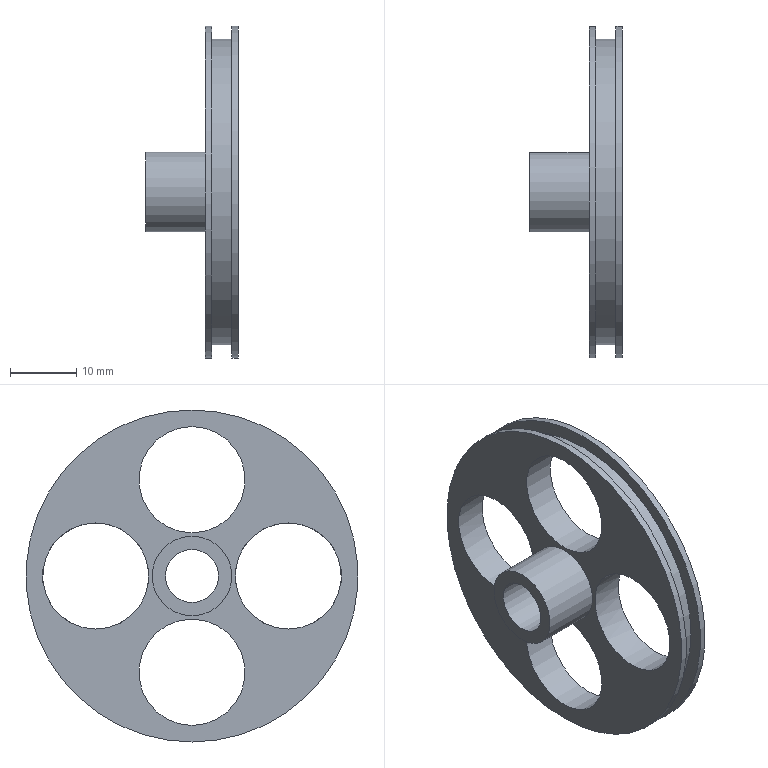Part | NX | features DATUM_CSYS 3, SKETCH 2, EXTRUDE 1, SWP104 1 | 1 solid | 14 faces | box 14 x 50 x 50 mm | volume 5206 mm3 | cylinder 9 | plane 5 | commonest cylinder face diameters 16 x4 50 x2 8 x1 12 x1 46 x1
STEP:
#1=CARTESIAN_POINT('',(-14.,0.,4.));
#2=VERTEX_POINT('',#1);
#3=CARTESIAN_POINT('',(-14.,0.,0.));
#4=DIRECTION('',(-1.,0.,0.));
#5=DIRECTION('',(0.,0.,1.));
#6=AXIS2_PLACEMENT_3D('',#3,#4,#5);
#7=CIRCLE('',#6,4.);
#8=EDGE_CURVE('',#2,#2,#7,.T.);
#9=ORIENTED_EDGE('',*,*,#8,.F.);
#10=EDGE_LOOP('',(#9));
#11=FACE_BOUND('',#10,.T.);
#12=CARTESIAN_POINT('',(-14.,0.,6.));
#13=VERTEX_POINT('',#12);
#14=CARTESIAN_POINT('',(-14.,0.,0.));
#15=DIRECTION('',(-1.,0.,0.));
#16=DIRECTION('',(0.,0.,1.));
#17=AXIS2_PLACEMENT_3D('',#14,#15,#16);
#18=CIRCLE('',#17,6.);
#19=EDGE_CURVE('',#13,#13,#18,.T.);
#20=ORIENTED_EDGE('',*,*,#19,.T.);
#21=EDGE_LOOP('',(#20));
#22=FACE_BOUND('',#21,.T.);
#23=CARTESIAN_POINT('',(-14.,6.,0.));
#24=DIRECTION('',(1.,0.,0.));
#25=DIRECTION('',(0.,0.,-1.));
#26=AXIS2_PLACEMENT_3D('',#23,#24,#25);
#27=PLANE('',#26);
#28=ADVANCED_FACE('',(#11,#22),#27,.F.);
#29=CARTESIAN_POINT('',(0.,0.,4.));
#30=VERTEX_POINT('',#29);
#31=CARTESIAN_POINT('',(0.,0.,0.));
#32=DIRECTION('',(-1.,0.,0.));
#33=DIRECTION('',(0.,0.,1.));
#34=AXIS2_PLACEMENT_3D('',#31,#32,#33);
#35=CIRCLE('',#34,4.);
#36=EDGE_CURVE('',#30,#30,#35,.T.);
#37=ORIENTED_EDGE('',*,*,#36,.F.);
#38=EDGE_LOOP('',(#37));
#39=FACE_BOUND('',#38,.T.);
#40=ORIENTED_EDGE('',*,*,#8,.T.);
#41=EDGE_LOOP('',(#40));
#42=FACE_BOUND('',#41,.T.);
#43=CARTESIAN_POINT('',(0.,0.,0.));
#44=DIRECTION('',(-1.,0.,0.));
#45=DIRECTION('',(0.,0.,1.));
#46=AXIS2_PLACEMENT_3D('',#43,#44,#45);
#47=CYLINDRICAL_SURFACE('',#46,4.);
#48=ADVANCED_FACE('',(#39,#42),#47,.F.);
#49=CARTESIAN_POINT('',(0.,6.5,0.));
#50=VERTEX_POINT('',#49);
#51=CARTESIAN_POINT('',(0.,14.5,0.));
#52=DIRECTION('',(-1.,0.,0.));
#53=DIRECTION('',(0.,-1.,0.));
#54=AXIS2_PLACEMENT_3D('',#51,#52,#53);
#55=CIRCLE('',#54,8.);
#56=EDGE_CURVE('',#50,#50,#55,.T.);
#57=ORIENTED_EDGE('',*,*,#56,.T.);
#58=EDGE_LOOP('',(#57));
#59=FACE_BOUND('',#58,.T.);
#60=CARTESIAN_POINT('',(0.,0.,-6.5));
#61=VERTEX_POINT('',#60);
#62=CARTESIAN_POINT('',(0.,0.,-14.5));
#63=DIRECTION('',(-1.,0.,0.));
#64=DIRECTION('',(0.,0.,1.));
#65=AXIS2_PLACEMENT_3D('',#62,#63,#64);
#66=CIRCLE('',#65,8.);
#67=EDGE_CURVE('',#61,#61,#66,.T.);
#68=ORIENTED_EDGE('',*,*,#67,.T.);
#69=EDGE_LOOP('',(#68));
#70=FACE_BOUND('',#69,.T.);
#71=CARTESIAN_POINT('',(0.,-6.5,0.));
#72=VERTEX_POINT('',#71);
#73=CARTESIAN_POINT('',(0.,-14.5,0.));
#74=DIRECTION('',(-1.,0.,0.));
#75=DIRECTION('',(0.,1.,0.));
#76=AXIS2_PLACEMENT_3D('',#73,#74,#75);
#77=CIRCLE('',#76,8.);
#78=EDGE_CURVE('',#72,#72,#77,.T.);
#79=ORIENTED_EDGE('',*,*,#78,.T.);
#80=EDGE_LOOP('',(#79));
#81=FACE_BOUND('',#80,.T.);
#82=CARTESIAN_POINT('',(0.,0.,6.5));
#83=VERTEX_POINT('',#82);
#84=CARTESIAN_POINT('',(0.,0.,14.5));
#85=DIRECTION('',(-1.,0.,0.));
#86=DIRECTION('',(0.,0.,-1.));
#87=AXIS2_PLACEMENT_3D('',#84,#85,#86);
#88=CIRCLE('',#87,8.);
#89=EDGE_CURVE('',#83,#83,#88,.T.);
#90=ORIENTED_EDGE('',*,*,#89,.T.);
#91=EDGE_LOOP('',(#90));
#92=FACE_BOUND('',#91,.T.);
#93=CARTESIAN_POINT('',(0.,0.,25.));
#94=VERTEX_POINT('',#93);
#95=CARTESIAN_POINT('',(0.,0.,0.));
#96=DIRECTION('',(-1.,0.,0.));
#97=DIRECTION('',(0.,0.,1.));
#98=AXIS2_PLACEMENT_3D('',#95,#96,#97);
#99=CIRCLE('',#98,25.);
#100=EDGE_CURVE('',#94,#94,#99,.T.);
#101=ORIENTED_EDGE('',*,*,#100,.F.);
#102=EDGE_LOOP('',(#101));
#103=FACE_BOUND('',#102,.T.);
#104=ORIENTED_EDGE('',*,*,#36,.T.);
#105=EDGE_LOOP('',(#104));
#106=FACE_BOUND('',#105,.T.);
#107=CARTESIAN_POINT('',(0.,4.,0.));
#108=DIRECTION('',(-1.,0.,0.));
#109=DIRECTION('',(0.,0.,1.));
#110=AXIS2_PLACEMENT_3D('',#107,#108,#109);
#111=PLANE('',#110);
#112=ADVANCED_FACE('',(#59,#70,#81,#92,#103,#106),#111,.F.);
#113=CARTESIAN_POINT('',(-1.,0.,25.));
#114=VERTEX_POINT('',#113);
#115=CARTESIAN_POINT('',(-1.,0.,0.));
#116=DIRECTION('',(-1.,0.,0.));
#117=DIRECTION('',(0.,0.,1.));
#118=AXIS2_PLACEMENT_3D('',#115,#116,#117);
#119=CIRCLE('',#118,25.);
#120=EDGE_CURVE('',#114,#114,#119,.T.);
#121=ORIENTED_EDGE('',*,*,#120,.F.);
#122=EDGE_LOOP('',(#121));
#123=FACE_BOUND('',#122,.T.);
#124=ORIENTED_EDGE('',*,*,#100,.T.);
#125=EDGE_LOOP('',(#124));
#126=FACE_BOUND('',#125,.T.);
#127=CARTESIAN_POINT('',(0.,0.,0.));
#128=DIRECTION('',(-1.,0.,0.));
#129=DIRECTION('',(0.,0.,1.));
#130=AXIS2_PLACEMENT_3D('',#127,#128,#129);
#131=CYLINDRICAL_SURFACE('',#130,25.);
#132=ADVANCED_FACE('',(#123,#126),#131,.T.);
#133=CARTESIAN_POINT('',(-1.,0.,23.));
#134=VERTEX_POINT('',#133);
#135=CARTESIAN_POINT('',(-1.,0.,0.));
#136=DIRECTION('',(-1.,0.,0.));
#137=DIRECTION('',(0.,0.,1.));
#138=AXIS2_PLACEMENT_3D('',#135,#136,#137);
#139=CIRCLE('',#138,23.);
#140=EDGE_CURVE('',#134,#134,#139,.T.);
#141=ORIENTED_EDGE('',*,*,#140,.F.);
#142=EDGE_LOOP('',(#141));
#143=FACE_BOUND('',#142,.T.);
#144=ORIENTED_EDGE('',*,*,#120,.T.);
#145=EDGE_LOOP('',(#144));
#146=FACE_BOUND('',#145,.T.);
#147=CARTESIAN_POINT('',(-1.,25.,0.));
#148=DIRECTION('',(1.,0.,0.));
#149=DIRECTION('',(0.,0.,-1.));
#150=AXIS2_PLACEMENT_3D('',#147,#148,#149);
#151=PLANE('',#150);
#152=ADVANCED_FACE('',(#143,#146),#151,.F.);
#153=CARTESIAN_POINT('',(-4.,0.,23.));
#154=VERTEX_POINT('',#153);
#155=CARTESIAN_POINT('',(-4.,0.,0.));
#156=DIRECTION('',(-1.,0.,0.));
#157=DIRECTION('',(0.,0.,1.));
#158=AXIS2_PLACEMENT_3D('',#155,#156,#157);
#159=CIRCLE('',#158,23.);
#160=EDGE_CURVE('',#154,#154,#159,.T.);
#161=ORIENTED_EDGE('',*,*,#160,.F.);
#162=EDGE_LOOP('',(#161));
#163=FACE_BOUND('',#162,.T.);
#164=ORIENTED_EDGE('',*,*,#140,.T.);
#165=EDGE_LOOP('',(#164));
#166=FACE_BOUND('',#165,.T.);
#167=CARTESIAN_POINT('',(0.,0.,0.));
#168=DIRECTION('',(-1.,0.,0.));
#169=DIRECTION('',(0.,0.,1.));
#170=AXIS2_PLACEMENT_3D('',#167,#168,#169);
#171=CYLINDRICAL_SURFACE('',#170,23.);
#172=ADVANCED_FACE('',(#163,#166),#171,.T.);
#173=CARTESIAN_POINT('',(-4.,0.,25.));
#174=VERTEX_POINT('',#173);
#175=CARTESIAN_POINT('',(-4.,0.,0.));
#176=DIRECTION('',(-1.,0.,0.));
#177=DIRECTION('',(0.,0.,1.));
#178=AXIS2_PLACEMENT_3D('',#175,#176,#177);
#179=CIRCLE('',#178,25.);
#180=EDGE_CURVE('',#174,#174,#179,.T.);
#181=ORIENTED_EDGE('',*,*,#180,.F.);
#182=EDGE_LOOP('',(#181));
#183=FACE_BOUND('',#182,.T.);
#184=ORIENTED_EDGE('',*,*,#160,.T.);
#185=EDGE_LOOP('',(#184));
#186=FACE_BOUND('',#185,.T.);
#187=CARTESIAN_POINT('',(-4.,23.,0.));
#188=DIRECTION('',(-1.,0.,0.));
#189=DIRECTION('',(0.,0.,1.));
#190=AXIS2_PLACEMENT_3D('',#187,#188,#189);
#191=PLANE('',#190);
#192=ADVANCED_FACE('',(#183,#186),#191,.F.);
#193=CARTESIAN_POINT('',(-5.,0.,25.));
#194=VERTEX_POINT('',#193);
#195=CARTESIAN_POINT('',(-5.,0.,0.));
#196=DIRECTION('',(-1.,0.,0.));
#197=DIRECTION('',(0.,0.,1.));
#198=AXIS2_PLACEMENT_3D('',#195,#196,#197);
#199=CIRCLE('',#198,25.);
#200=EDGE_CURVE('',#194,#194,#199,.T.);
#201=ORIENTED_EDGE('',*,*,#200,.F.);
#202=EDGE_LOOP('',(#201));
#203=FACE_BOUND('',#202,.T.);
#204=ORIENTED_EDGE('',*,*,#180,.T.);
#205=EDGE_LOOP('',(#204));
#206=FACE_BOUND('',#205,.T.);
#207=CARTESIAN_POINT('',(0.,0.,0.));
#208=DIRECTION('',(-1.,0.,0.));
#209=DIRECTION('',(0.,0.,1.));
#210=AXIS2_PLACEMENT_3D('',#207,#208,#209);
#211=CYLINDRICAL_SURFACE('',#210,25.);
#212=ADVANCED_FACE('',(#203,#206),#211,.T.);
#213=CARTESIAN_POINT('',(-5.,14.5,-8.));
#214=VERTEX_POINT('',#213);
#215=CARTESIAN_POINT('',(-5.,14.5,0.));
#216=DIRECTION('',(1.,0.,0.));
#217=DIRECTION('',(0.,0.,-1.));
#218=AXIS2_PLACEMENT_3D('',#215,#216,#217);
#219=CIRCLE('',#218,8.);
#220=EDGE_CURVE('',#214,#214,#219,.F.);
#221=ORIENTED_EDGE('',*,*,#220,.F.);
#222=EDGE_LOOP('',(#221));
#223=FACE_BOUND('',#222,.T.);
#224=CARTESIAN_POINT('',(-5.,0.,-22.5));
#225=VERTEX_POINT('',#224);
#226=CARTESIAN_POINT('',(-5.,0.,-14.5));
#227=DIRECTION('',(1.,0.,0.));
#228=DIRECTION('',(0.,0.,-1.));
#229=AXIS2_PLACEMENT_3D('',#226,#227,#228);
#230=CIRCLE('',#229,8.);
#231=EDGE_CURVE('',#225,#225,#230,.F.);
#232=ORIENTED_EDGE('',*,*,#231,.F.);
#233=EDGE_LOOP('',(#232));
#234=FACE_BOUND('',#233,.T.);
#235=CARTESIAN_POINT('',(-5.,-14.5,-8.));
#236=VERTEX_POINT('',#235);
#237=CARTESIAN_POINT('',(-5.,-14.5,0.));
#238=DIRECTION('',(1.,0.,0.));
#239=DIRECTION('',(0.,0.,-1.));
#240=AXIS2_PLACEMENT_3D('',#237,#238,#239);
#241=CIRCLE('',#240,8.);
#242=EDGE_CURVE('',#236,#236,#241,.F.);
#243=ORIENTED_EDGE('',*,*,#242,.F.);
#244=EDGE_LOOP('',(#243));
#245=FACE_BOUND('',#244,.T.);
#246=CARTESIAN_POINT('',(-5.,0.,6.5));
#247=VERTEX_POINT('',#246);
#248=CARTESIAN_POINT('',(-5.,0.,14.5));
#249=DIRECTION('',(1.,0.,0.));
#250=DIRECTION('',(0.,0.,-1.));
#251=AXIS2_PLACEMENT_3D('',#248,#249,#250);
#252=CIRCLE('',#251,8.);
#253=EDGE_CURVE('',#247,#247,#252,.F.);
#254=ORIENTED_EDGE('',*,*,#253,.F.);
#255=EDGE_LOOP('',(#254));
#256=FACE_BOUND('',#255,.T.);
#257=CARTESIAN_POINT('',(-5.,0.,6.));
#258=VERTEX_POINT('',#257);
#259=CARTESIAN_POINT('',(-5.,0.,0.));
#260=DIRECTION('',(-1.,0.,0.));
#261=DIRECTION('',(0.,0.,1.));
#262=AXIS2_PLACEMENT_3D('',#259,#260,#261);
#263=CIRCLE('',#262,6.);
#264=EDGE_CURVE('',#258,#258,#263,.T.);
#265=ORIENTED_EDGE('',*,*,#264,.F.);
#266=EDGE_LOOP('',(#265));
#267=FACE_BOUND('',#266,.T.);
#268=ORIENTED_EDGE('',*,*,#200,.T.);
#269=EDGE_LOOP('',(#268));
#270=FACE_BOUND('',#269,.T.);
#271=CARTESIAN_POINT('',(-5.,25.,0.));
#272=DIRECTION('',(1.,0.,0.));
#273=DIRECTION('',(0.,0.,-1.));
#274=AXIS2_PLACEMENT_3D('',#271,#272,#273);
#275=PLANE('',#274);
#276=ADVANCED_FACE('',(#223,#234,#245,#256,#267,#270),#275,.F.);
#277=ORIENTED_EDGE('',*,*,#19,.F.);
#278=EDGE_LOOP('',(#277));
#279=FACE_BOUND('',#278,.T.);
#280=ORIENTED_EDGE('',*,*,#264,.T.);
#281=EDGE_LOOP('',(#280));
#282=FACE_BOUND('',#281,.T.);
#283=CARTESIAN_POINT('',(0.,0.,0.));
#284=DIRECTION('',(-1.,0.,0.));
#285=DIRECTION('',(0.,0.,1.));
#286=AXIS2_PLACEMENT_3D('',#283,#284,#285);
#287=CYLINDRICAL_SURFACE('',#286,6.);
#288=ADVANCED_FACE('',(#279,#282),#287,.T.);
#289=ORIENTED_EDGE('',*,*,#89,.F.);
#290=EDGE_LOOP('',(#289));
#291=FACE_BOUND('',#290,.T.);
#292=ORIENTED_EDGE('',*,*,#253,.T.);
#293=EDGE_LOOP('',(#292));
#294=FACE_BOUND('',#293,.T.);
#295=CARTESIAN_POINT('',(-10.,0.,14.5));
#296=DIRECTION('',(1.,0.,0.));
#297=DIRECTION('',(0.,0.,-1.));
#298=AXIS2_PLACEMENT_3D('',#295,#296,#297);
#299=CYLINDRICAL_SURFACE('',#298,8.);
#300=ADVANCED_FACE('',(#291,#294),#299,.F.);
#301=ORIENTED_EDGE('',*,*,#78,.F.);
#302=EDGE_LOOP('',(#301));
#303=FACE_BOUND('',#302,.T.);
#304=ORIENTED_EDGE('',*,*,#242,.T.);
#305=EDGE_LOOP('',(#304));
#306=FACE_BOUND('',#305,.T.);
#307=CARTESIAN_POINT('',(-10.,-14.5,0.));
#308=DIRECTION('',(1.,0.,0.));
#309=DIRECTION('',(0.,0.,-1.));
#310=AXIS2_PLACEMENT_3D('',#307,#308,#309);
#311=CYLINDRICAL_SURFACE('',#310,8.);
#312=ADVANCED_FACE('',(#303,#306),#311,.F.);
#313=ORIENTED_EDGE('',*,*,#67,.F.);
#314=EDGE_LOOP('',(#313));
#315=FACE_BOUND('',#314,.T.);
#316=ORIENTED_EDGE('',*,*,#231,.T.);
#317=EDGE_LOOP('',(#316));
#318=FACE_BOUND('',#317,.T.);
#319=CARTESIAN_POINT('',(-10.,0.,-14.5));
#320=DIRECTION('',(1.,0.,0.));
#321=DIRECTION('',(0.,0.,-1.));
#322=AXIS2_PLACEMENT_3D('',#319,#320,#321);
#323=CYLINDRICAL_SURFACE('',#322,8.);
#324=ADVANCED_FACE('',(#315,#318),#323,.F.);
#325=ORIENTED_EDGE('',*,*,#56,.F.);
#326=EDGE_LOOP('',(#325));
#327=FACE_BOUND('',#326,.T.);
#328=ORIENTED_EDGE('',*,*,#220,.T.);
#329=EDGE_LOOP('',(#328));
#330=FACE_BOUND('',#329,.T.);
#331=CARTESIAN_POINT('',(-10.,14.5,0.));
#332=DIRECTION('',(1.,0.,0.));
#333=DIRECTION('',(0.,0.,-1.));
#334=AXIS2_PLACEMENT_3D('',#331,#332,#333);
#335=CYLINDRICAL_SURFACE('',#334,8.);
#336=ADVANCED_FACE('',(#327,#330),#335,.F.);
#337=CLOSED_SHELL('',(#28,#48,#112,#132,#152,#172,#192,#212,#276,#288,#300,#312,#324,#336));
#338=MANIFOLD_SOLID_BREP('',#337);
#339=(LENGTH_UNIT()NAMED_UNIT(*)SI_UNIT(.MILLI.,.METRE.));
#340=UNCERTAINTY_MEASURE_WITH_UNIT(LENGTH_MEASURE(0.00001),#339,'','');
#341=(NAMED_UNIT(*)PLANE_ANGLE_UNIT()SI_UNIT($,.RADIAN.));
#342=(NAMED_UNIT(*)SI_UNIT($,.STERADIAN.)SOLID_ANGLE_UNIT());
#343=(GEOMETRIC_REPRESENTATION_CONTEXT(3)GLOBAL_UNCERTAINTY_ASSIGNED_CONTEXT((#340))GLOBAL_UNIT_ASSIGNED_CONTEXT((#339,#341,#342))REPRESENTATION_CONTEXT('',''));
#344=ADVANCED_BREP_SHAPE_REPRESENTATION('',(#338),#343);